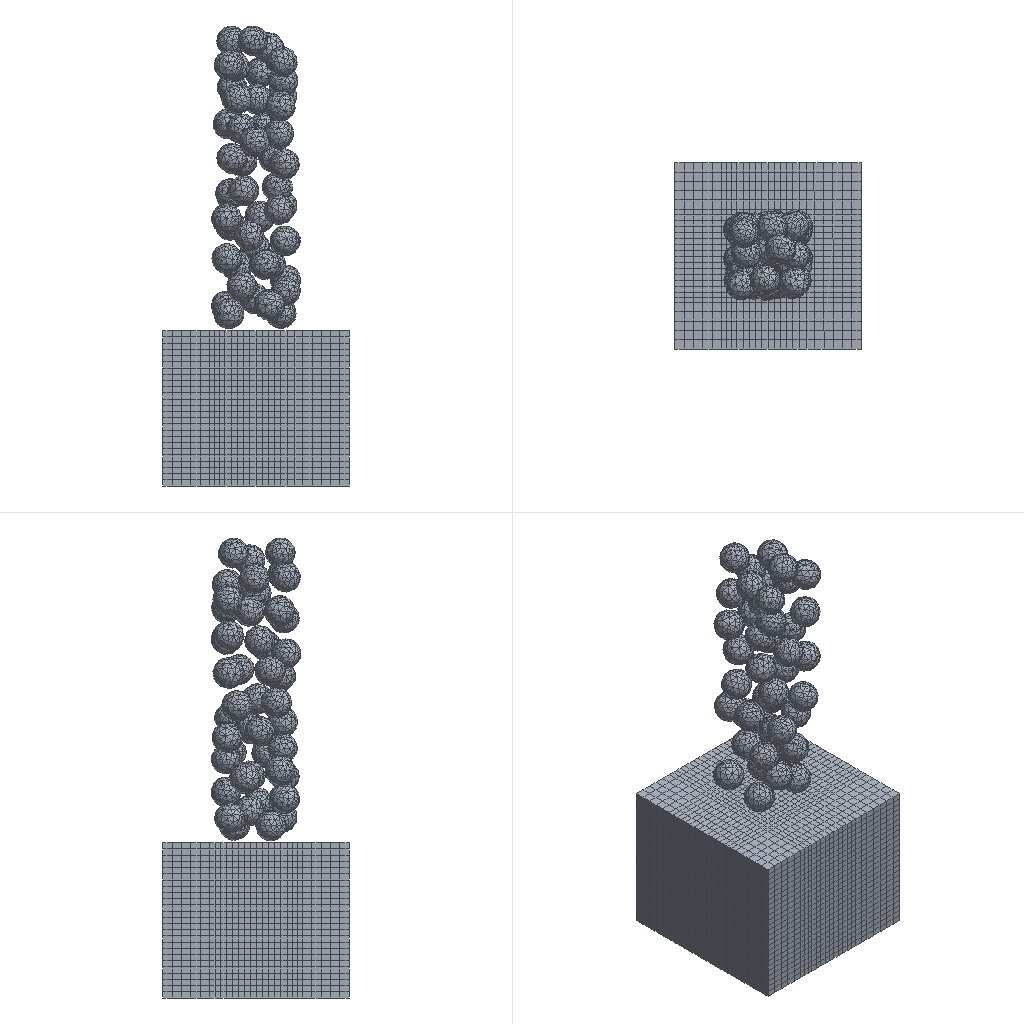Simulation study | abaqus
Set-up summary:
category,name,step,type,value,unit,region
solver,abaqus
solver,version,,,Abaqus/Explicit 2020
units,not stated in the deck,,not stated
analysis,deck,,transient,transient
load_step,Step-1,Step-1,transient
load_step,requested,,,1
mesh,nodes,,,63515
mesh,elements,,,43155
element_type,C3D10,,solid,26905
element_type,C3D8R,,solid,16250
load,load commands in deck,,count,1
bc,support commands in deck,,count,1
material,KELI,,in results
material,WORK,,in results
check,setup vs results,,match,"per instance, exact: element labels, types and connectivity; labels of the nodes the elements use; coordinates of those nodes at SINGLE_PRECISION in 1 of 2 instance(s)"
Abaqus input file, long lists of numbers shortened:
*Heading
** Job name: Job-1 Model name: Model-1
** Generated by: Abaqus/CAE 2020
*Preprint, echo=NO, model=NO, history=NO, contact=NO
**
** PARTS
**
*Part, name=Parricles
*Node
      1,   117.035,   95.266,   62.994
      2,   128.712,   48.506,   65.817
** (45261 more lines like these left out)
*Element, type=C3D10
  1, 4315, 4316, 4317, 4318, 7094, 7093, 7092, 7096, 7095, 7097
  2, 4318, 4316, 4319,  439, 7095, 7099, 7098, 7101, 7100, 7102
** (26903 more lines like these left out)
*Nset, nset=Set-3, generate
     1,  45263,      1
*Elset, elset=Set-3, generate
     1,  26905,      1
** Section: keli
*Solid Section, elset=Set-3, material=keli
,
*End Part
**
*Part, name=work
*Node
      1,          75.,        -200.,           0.
      2,          75.,        -200.,         250.
** (18250 more lines like these left out)
*Element, type=C3D8R
   1,  206, 1693, 8173, 1621,    1,   77, 1429,  132
   2, 1693, 1694, 8174, 8173,   77,   78, 1430, 1429
** (16248 more lines like these left out)
*Nset, nset=Set-3, generate
     1,  18252,      1
*Elset, elset=Set-3, generate
     1,  16250,      1
** Section: work
*Solid Section, elset=Set-3, material=work
,
*End Part
**
**
** ASSEMBLY
**
*Assembly, name=Assembly
**
*Instance, name=Parricles-1, part=Parricles
         75.,        -225.,         250.
*End Instance
**
*Instance, name=work-1, part=work
*End Instance
**
*Node
      1,   198.642,  -138.2,   273.508
*Nset, nset=Set-3, instance=work-1
    1,    4,    5,    8,    9,   11,   13,   15,   16,   19,   20,   23,   26,   27,   29,   30
   35,   36,   37,   40,   41,   43,   44,   47,   49,   52,   54,   55,   58,   59,   62,   64
** (42 more lines like these left out)
*Elset, elset=Set-3, instance=work-1
     1,    26,    51,    76,   101,   126,   151,   176,   201,   226,   251,   276,   301,   326,   351,   376
   401,   426,   451,   476,   501,   526,   551,   576,   601,   626,   651,   676,   701,   726,   751,   776
** (39 more lines like these left out)
*Nset, nset=Set-4, instance=Parricles-1, generate
     1,  45263,      1
*Nset, nset=Set-4
 1,
*Elset, elset=Set-4, instance=Parricles-1, generate
     1,  26905,      1
*Nset, nset=Set-5, instance=Parricles-1, generate
     1,  45263,      1
*Elset, elset=Set-5, instance=Parricles-1, generate
     1,  26905,      1
*Nset, nset=b_Set-1, instance=Parricles-1, generate
     1,  45263,      1
*Elset, elset=b_Set-1, instance=Parricles-1, generate
     1,  26905,      1
*Nset, nset=_PickedSet144, internal
 1,
** Constraint: Constraint-1
*Rigid Body, ref node=_PickedSet144, elset=b_Set-1
*End Assembly
**
** MATERIALS
**
*Material, name=keli
*Density
 3.86e-09,
*Elastic
330000., 0.27
*Material, name=work
*Density
 4.4e-09,
*Elastic
114000., 0.34
*Plastic, hardening=JOHNSON COOK
1098.,1092., 0.93,  1.1,1933., 293.
**
** INTERACTION PROPERTIES
**
*Surface Interaction, name=IntProp-1
*Friction
 0.2,
*Surface Behavior, pressure-overclosure=HARD
**
** BOUNDARY CONDITIONS
**
** Name: BC-1 Type: 对称/反对称/完全固定
*Boundary
Set-3, ENCASTRE
**
** PREDEFINED FIELDS
**
** Name: Predefined Field-1   Type: Velocity
*Initial Conditions, type=VELOCITY
Set-4, 1, 0.
Set-4, 2, 0.
Set-4, 3, -5000.
**
** INTERACTIONS
**
** Interaction: Int-1
*Contact, op=NEW
*Contact Inclusions, ALL EXTERIOR
*Contact Property Assignment
 ,  , IntProp-1
** ----------------------------------------------------------------
**
** STEP: Step-1
**
*Step, name=Step-1, nlgeom=YES
*Dynamic, Explicit
, 0.001
*Bulk Viscosity
0.06, 1.2
** Mass Scaling: Semi-Automatic
**               Whole Model
*Fixed Mass Scaling, factor=1000.
**
** OUTPUT REQUESTS
**
*Restart, write, number interval=1, time marks=NO
**
** FIELD OUTPUT: F-Output-1
**
*Output, field, number interval=100
*Node Output
A, RF, RT, U, V
*Element Output, directions=YES
E, EVF, LE, MISES, PE, PEEQ, PEEQMAX, PEEQT, PEEQVAVG, PEMAG, PEQC, PEVAVG, S, SVAVG
*Contact Output
CDISP, CSTRESS
**
** HISTORY OUTPUT: H-Output-1
**
*Output, history, variable=PRESELECT
*End Step
Results summary:
result,step,Step-1,partial,increments=22 time=0.0006635/0.001
result,analysis,,,transient
result,last_loadstep,,,1
result,primary field,,,U